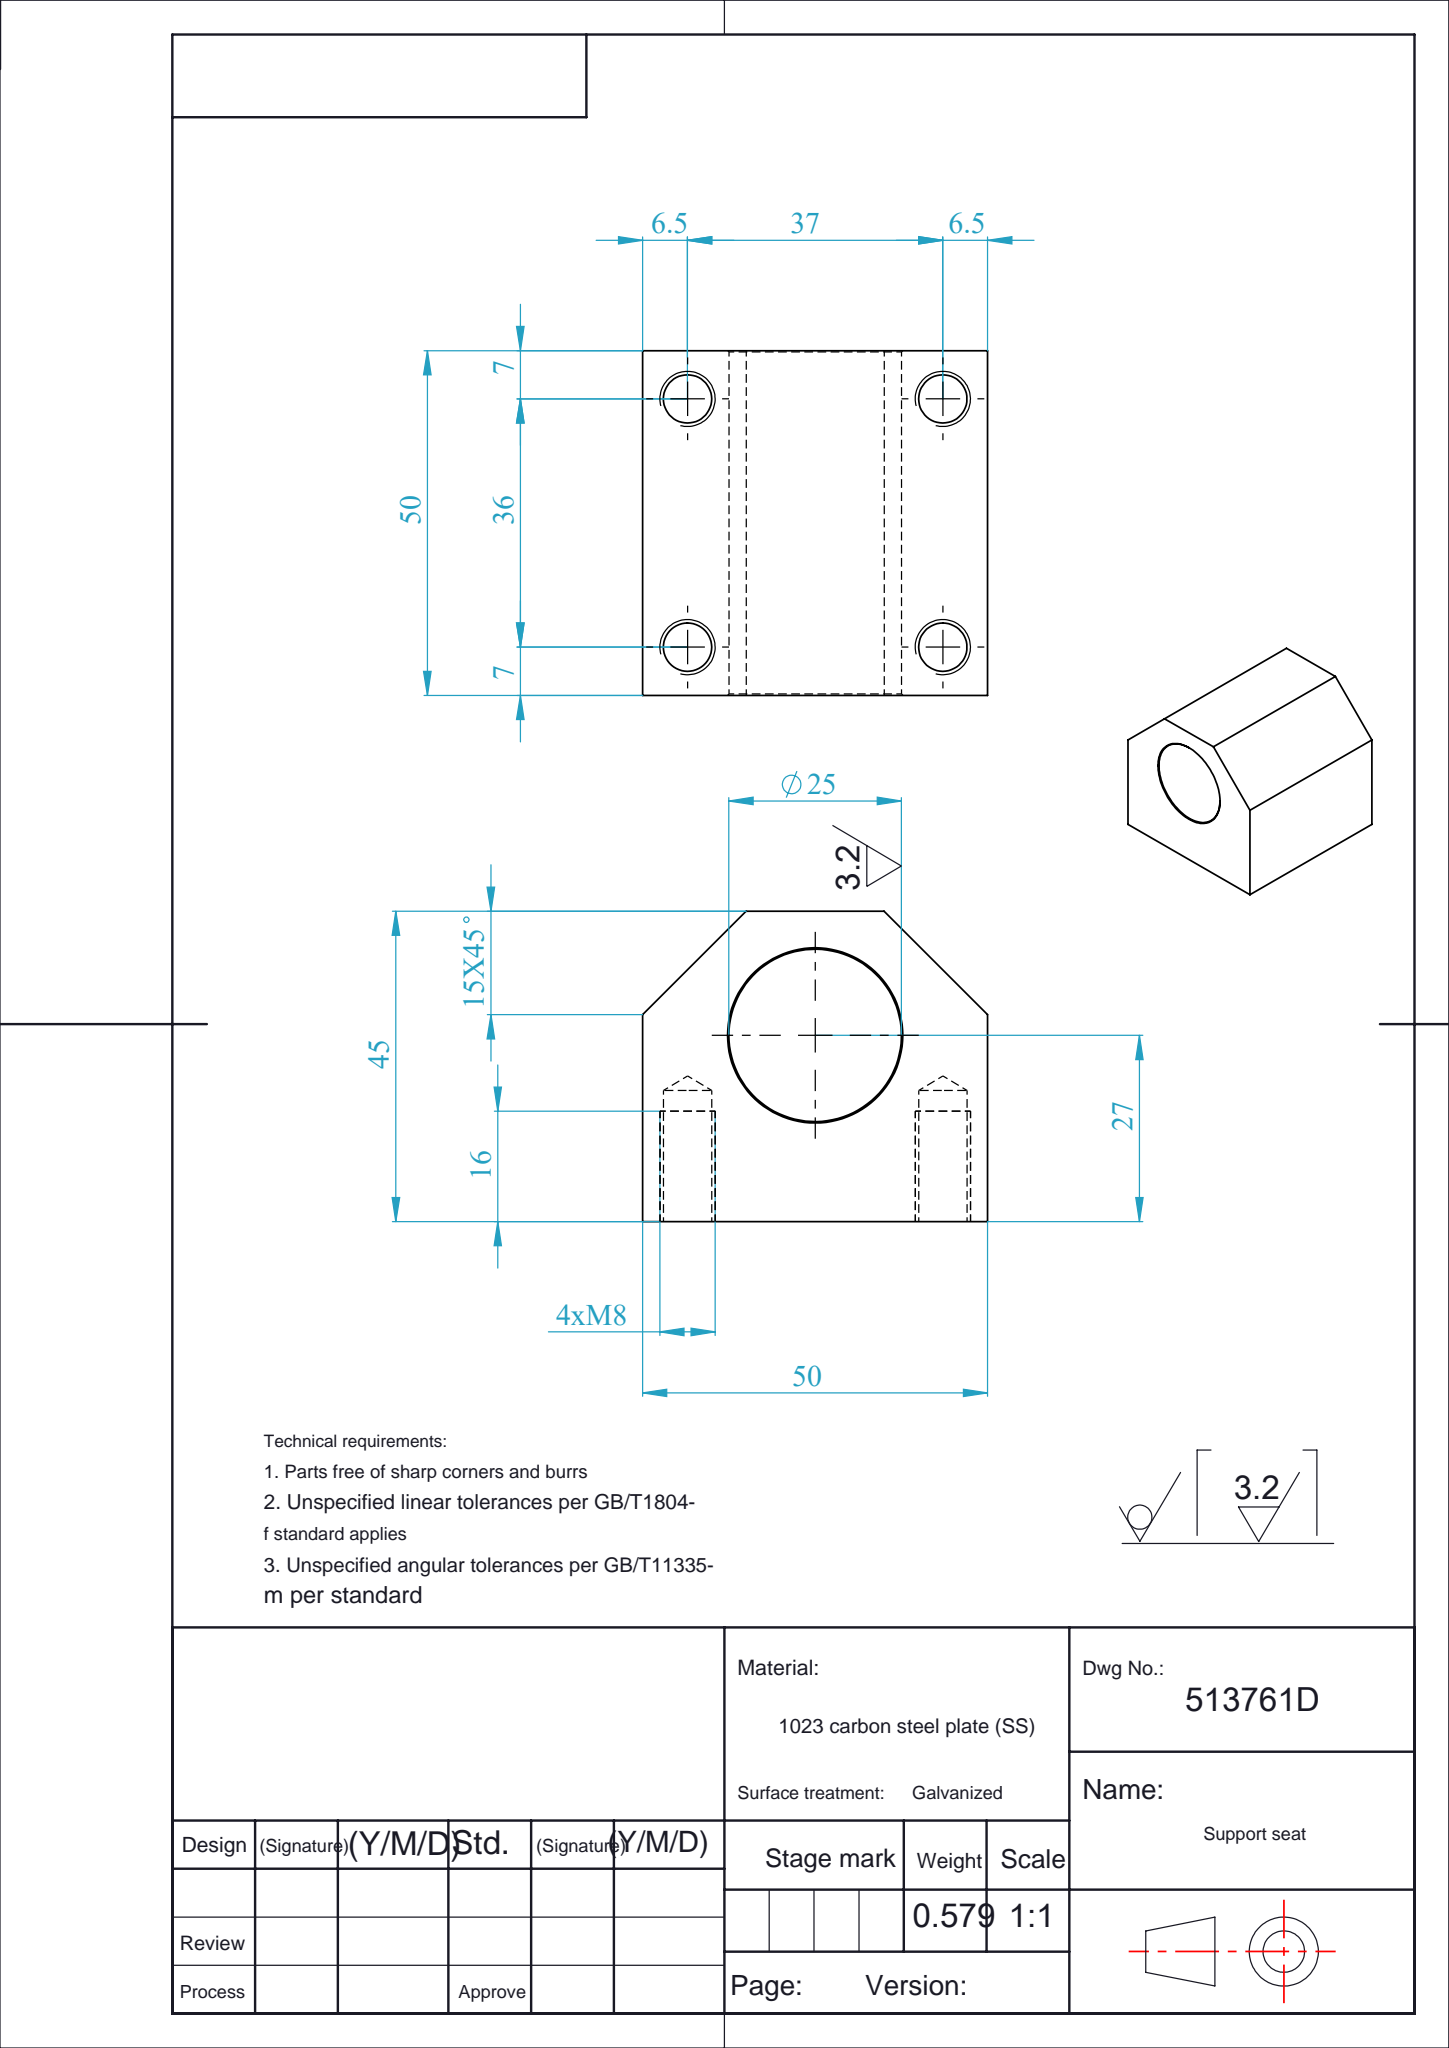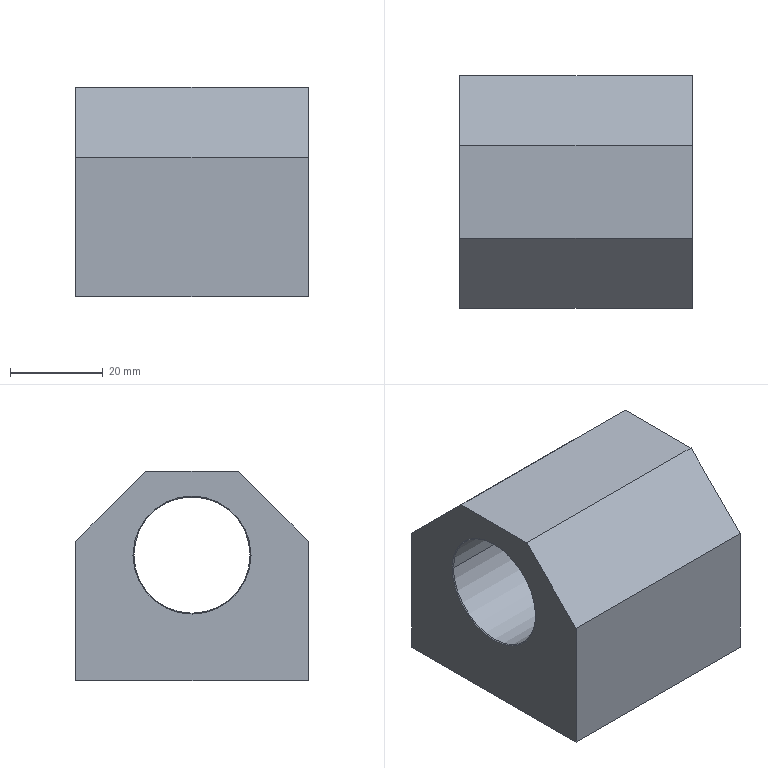Part | SolidWorks | features Chamfer 3, Extrusion 1, HoleWzd 1, ICE 1 | 1 solid | 30 faces | box 50 x 50 x 45 mm | volume 73670 mm3 | cone 12 | cylinder 10 | plane 8 | commonest cylinder face diameters 7 x8 25 x2
STEP:
#1=CARTESIAN_POINT('',(-24.8,12.5,27.));
#2=VERTEX_POINT('',#1);
#3=CARTESIAN_POINT('',(-24.8,-12.5,27.));
#4=VERTEX_POINT('',#3);
#5=CARTESIAN_POINT('',(-24.8,0.,27.));
#6=DIRECTION('',(-1.,0.,0.));
#7=DIRECTION('',(0.,1.,0.));
#8=AXIS2_PLACEMENT_3D('',#5,#6,#7);
#9=CIRCLE('',#8,12.5);
#10=EDGE_CURVE('',#2,#4,#9,.T.);
#11=ORIENTED_EDGE('',*,*,#10,.F.);
#12=CARTESIAN_POINT('',(-25.,12.7,27.));
#13=VERTEX_POINT('',#12);
#14=CARTESIAN_POINT('',(-25.,12.7,27.));
#15=DIRECTION('',(-0.7071,0.7071,0.));
#16=VECTOR('',#15,1000.);
#17=LINE('',#14,#16);
#18=EDGE_CURVE('',#2,#13,#17,.T.);
#19=ORIENTED_EDGE('',*,*,#18,.T.);
#20=CARTESIAN_POINT('',(-25.,-12.7,27.));
#21=VERTEX_POINT('',#20);
#22=CARTESIAN_POINT('',(-25.,0.,27.));
#23=DIRECTION('',(1.,0.,0.));
#24=DIRECTION('',(0.,1.,0.));
#25=AXIS2_PLACEMENT_3D('',#22,#23,#24);
#26=CIRCLE('',#25,12.7);
#27=EDGE_CURVE('',#21,#13,#26,.T.);
#28=ORIENTED_EDGE('',*,*,#27,.F.);
#29=CARTESIAN_POINT('',(-25.,-12.7,27.));
#30=DIRECTION('',(-0.7071,-0.7071,0.));
#31=VECTOR('',#30,1000.);
#32=LINE('',#29,#31);
#33=EDGE_CURVE('',#4,#21,#32,.T.);
#34=ORIENTED_EDGE('',*,*,#33,.F.);
#35=EDGE_LOOP('',(#11,#19,#28,#34));
#36=FACE_OUTER_BOUND('',#35,.T.);
#37=CARTESIAN_POINT('',(-25.,0.,27.));
#38=DIRECTION('',(-1.,0.,0.));
#39=DIRECTION('',(0.,-1.,0.));
#40=AXIS2_PLACEMENT_3D('',#37,#38,#39);
#41=CONICAL_SURFACE('',#40,12.7,0.7854);
#42=ADVANCED_FACE('',(#36),#41,.F.);
#43=CARTESIAN_POINT('',(24.8,-12.5,27.));
#44=VERTEX_POINT('',#43);
#45=CARTESIAN_POINT('',(24.8,12.5,27.));
#46=VERTEX_POINT('',#45);
#47=CARTESIAN_POINT('',(24.8,0.,27.));
#48=DIRECTION('',(1.,0.,0.));
#49=DIRECTION('',(0.,-1.,0.));
#50=AXIS2_PLACEMENT_3D('',#47,#48,#49);
#51=CIRCLE('',#50,12.5);
#52=EDGE_CURVE('',#44,#46,#51,.T.);
#53=ORIENTED_EDGE('',*,*,#52,.F.);
#54=CARTESIAN_POINT('',(25.,-12.7,27.));
#55=VERTEX_POINT('',#54);
#56=CARTESIAN_POINT('',(24.8,-12.5,27.));
#57=DIRECTION('',(0.7071,-0.7071,0.));
#58=VECTOR('',#57,1000.);
#59=LINE('',#56,#58);
#60=EDGE_CURVE('',#44,#55,#59,.T.);
#61=ORIENTED_EDGE('',*,*,#60,.T.);
#62=CARTESIAN_POINT('',(25.,12.7,27.));
#63=VERTEX_POINT('',#62);
#64=CARTESIAN_POINT('',(25.,0.,27.));
#65=DIRECTION('',(-1.,0.,0.));
#66=DIRECTION('',(0.,-1.,0.));
#67=AXIS2_PLACEMENT_3D('',#64,#65,#66);
#68=CIRCLE('',#67,12.7);
#69=EDGE_CURVE('',#63,#55,#68,.T.);
#70=ORIENTED_EDGE('',*,*,#69,.F.);
#71=CARTESIAN_POINT('',(24.8,12.5,27.));
#72=DIRECTION('',(0.7071,0.7071,0.));
#73=VECTOR('',#72,1000.);
#74=LINE('',#71,#73);
#75=EDGE_CURVE('',#46,#63,#74,.T.);
#76=ORIENTED_EDGE('',*,*,#75,.F.);
#77=EDGE_LOOP('',(#53,#61,#70,#76));
#78=FACE_OUTER_BOUND('',#77,.T.);
#79=CARTESIAN_POINT('',(24.8,0.,27.));
#80=DIRECTION('',(1.,0.,0.));
#81=DIRECTION('',(0.,1.,0.));
#82=AXIS2_PLACEMENT_3D('',#79,#80,#81);
#83=CONICAL_SURFACE('',#82,12.5,0.7854);
#84=ADVANCED_FACE('',(#78),#83,.F.);
#85=CARTESIAN_POINT('',(21.5,18.5,19.));
#86=VERTEX_POINT('',#85);
#87=CARTESIAN_POINT('',(14.5,18.5,19.));
#88=VERTEX_POINT('',#87);
#89=CARTESIAN_POINT('',(18.,18.5,19.));
#90=DIRECTION('',(0.,0.,-1.));
#91=DIRECTION('',(-1.,0.,0.));
#92=AXIS2_PLACEMENT_3D('',#89,#90,#91);
#93=CIRCLE('',#92,3.5);
#94=EDGE_CURVE('',#86,#88,#93,.T.);
#95=ORIENTED_EDGE('',*,*,#94,.F.);
#96=CARTESIAN_POINT('',(21.5,18.5,0.));
#97=VERTEX_POINT('',#96);
#98=CARTESIAN_POINT('',(21.5,18.5,0.));
#99=DIRECTION('',(0.,0.,-1.));
#100=VECTOR('',#99,1000.);
#101=LINE('',#98,#100);
#102=EDGE_CURVE('',#86,#97,#101,.T.);
#103=ORIENTED_EDGE('',*,*,#102,.T.);
#104=CARTESIAN_POINT('',(14.5,18.5,0.));
#105=VERTEX_POINT('',#104);
#106=CARTESIAN_POINT('',(18.,18.5,0.));
#107=DIRECTION('',(0.,0.,-1.));
#108=DIRECTION('',(-1.,0.,0.));
#109=AXIS2_PLACEMENT_3D('',#106,#107,#108);
#110=CIRCLE('',#109,3.5);
#111=EDGE_CURVE('',#97,#105,#110,.T.);
#112=ORIENTED_EDGE('',*,*,#111,.T.);
#113=CARTESIAN_POINT('',(14.5,18.5,0.));
#114=DIRECTION('',(0.,0.,-1.));
#115=VECTOR('',#114,1000.);
#116=LINE('',#113,#115);
#117=EDGE_CURVE('',#88,#105,#116,.T.);
#118=ORIENTED_EDGE('',*,*,#117,.F.);
#119=EDGE_LOOP('',(#95,#103,#112,#118));
#120=FACE_OUTER_BOUND('',#119,.T.);
#121=CARTESIAN_POINT('',(18.,18.5,0.));
#122=DIRECTION('',(0.,0.,-1.));
#123=DIRECTION('',(-1.,0.,0.));
#124=AXIS2_PLACEMENT_3D('',#121,#122,#123);
#125=CYLINDRICAL_SURFACE('',#124,3.5);
#126=ADVANCED_FACE('',(#120),#125,.F.);
#127=CARTESIAN_POINT('',(18.,18.5,21.103));
#128=VERTEX_POINT('',#127);
#129=CARTESIAN_POINT('',(14.5,18.5,19.));
#130=DIRECTION('',(-0.8572,0.,-0.515));
#131=VECTOR('',#130,1000.);
#132=LINE('',#129,#131);
#133=EDGE_CURVE('',#128,#88,#132,.T.);
#134=ORIENTED_EDGE('',*,*,#133,.F.);
#135=CARTESIAN_POINT('',(21.5,18.5,19.));
#136=DIRECTION('',(0.8572,0.,-0.515));
#137=VECTOR('',#136,1000.);
#138=LINE('',#135,#137);
#139=EDGE_CURVE('',#128,#86,#138,.T.);
#140=ORIENTED_EDGE('',*,*,#139,.T.);
#141=ORIENTED_EDGE('',*,*,#94,.T.);
#142=EDGE_LOOP('',(#134,#140,#141));
#143=FACE_OUTER_BOUND('',#142,.T.);
#144=CARTESIAN_POINT('',(18.,18.5,19.));
#145=DIRECTION('',(0.,0.,-1.));
#146=DIRECTION('',(-1.,0.,0.));
#147=AXIS2_PLACEMENT_3D('',#144,#145,#146);
#148=CONICAL_SURFACE('',#147,3.5,1.03);
#149=ADVANCED_FACE('',(#143),#148,.F.);
#150=CARTESIAN_POINT('',(-14.5,18.5,19.));
#151=VERTEX_POINT('',#150);
#152=CARTESIAN_POINT('',(-21.5,18.5,19.));
#153=VERTEX_POINT('',#152);
#154=CARTESIAN_POINT('',(-18.,18.5,19.));
#155=DIRECTION('',(0.,0.,-1.));
#156=DIRECTION('',(-1.,0.,0.));
#157=AXIS2_PLACEMENT_3D('',#154,#155,#156);
#158=CIRCLE('',#157,3.5);
#159=EDGE_CURVE('',#151,#153,#158,.T.);
#160=ORIENTED_EDGE('',*,*,#159,.F.);
#161=CARTESIAN_POINT('',(-14.5,18.5,0.));
#162=VERTEX_POINT('',#161);
#163=CARTESIAN_POINT('',(-14.5,18.5,0.));
#164=DIRECTION('',(0.,0.,-1.));
#165=VECTOR('',#164,1000.);
#166=LINE('',#163,#165);
#167=EDGE_CURVE('',#151,#162,#166,.T.);
#168=ORIENTED_EDGE('',*,*,#167,.T.);
#169=CARTESIAN_POINT('',(-21.5,18.5,0.));
#170=VERTEX_POINT('',#169);
#171=CARTESIAN_POINT('',(-18.,18.5,0.));
#172=DIRECTION('',(0.,0.,-1.));
#173=DIRECTION('',(-1.,0.,0.));
#174=AXIS2_PLACEMENT_3D('',#171,#172,#173);
#175=CIRCLE('',#174,3.5);
#176=EDGE_CURVE('',#162,#170,#175,.T.);
#177=ORIENTED_EDGE('',*,*,#176,.T.);
#178=CARTESIAN_POINT('',(-21.5,18.5,0.));
#179=DIRECTION('',(0.,0.,-1.));
#180=VECTOR('',#179,1000.);
#181=LINE('',#178,#180);
#182=EDGE_CURVE('',#153,#170,#181,.T.);
#183=ORIENTED_EDGE('',*,*,#182,.F.);
#184=EDGE_LOOP('',(#160,#168,#177,#183));
#185=FACE_OUTER_BOUND('',#184,.T.);
#186=CARTESIAN_POINT('',(-18.,18.5,0.));
#187=DIRECTION('',(0.,0.,-1.));
#188=DIRECTION('',(-1.,0.,0.));
#189=AXIS2_PLACEMENT_3D('',#186,#187,#188);
#190=CYLINDRICAL_SURFACE('',#189,3.5);
#191=ADVANCED_FACE('',(#185),#190,.F.);
#192=CARTESIAN_POINT('',(-18.,18.5,21.103));
#193=VERTEX_POINT('',#192);
#194=CARTESIAN_POINT('',(-21.5,18.5,19.));
#195=DIRECTION('',(-0.8572,0.,-0.515));
#196=VECTOR('',#195,1000.);
#197=LINE('',#194,#196);
#198=EDGE_CURVE('',#193,#153,#197,.T.);
#199=ORIENTED_EDGE('',*,*,#198,.F.);
#200=CARTESIAN_POINT('',(-14.5,18.5,19.));
#201=DIRECTION('',(0.8572,0.,-0.515));
#202=VECTOR('',#201,1000.);
#203=LINE('',#200,#202);
#204=EDGE_CURVE('',#193,#151,#203,.T.);
#205=ORIENTED_EDGE('',*,*,#204,.T.);
#206=ORIENTED_EDGE('',*,*,#159,.T.);
#207=EDGE_LOOP('',(#199,#205,#206));
#208=FACE_OUTER_BOUND('',#207,.T.);
#209=CARTESIAN_POINT('',(-18.,18.5,19.));
#210=DIRECTION('',(0.,0.,-1.));
#211=DIRECTION('',(-1.,0.,0.));
#212=AXIS2_PLACEMENT_3D('',#209,#210,#211);
#213=CONICAL_SURFACE('',#212,3.5,1.03);
#214=ADVANCED_FACE('',(#208),#213,.F.);
#215=CARTESIAN_POINT('',(-14.5,-18.5,19.));
#216=VERTEX_POINT('',#215);
#217=CARTESIAN_POINT('',(-21.5,-18.5,19.));
#218=VERTEX_POINT('',#217);
#219=CARTESIAN_POINT('',(-18.,-18.5,19.));
#220=DIRECTION('',(0.,0.,-1.));
#221=DIRECTION('',(-1.,0.,0.));
#222=AXIS2_PLACEMENT_3D('',#219,#220,#221);
#223=CIRCLE('',#222,3.5);
#224=EDGE_CURVE('',#216,#218,#223,.T.);
#225=ORIENTED_EDGE('',*,*,#224,.F.);
#226=CARTESIAN_POINT('',(-14.5,-18.5,0.));
#227=VERTEX_POINT('',#226);
#228=CARTESIAN_POINT('',(-14.5,-18.5,0.));
#229=DIRECTION('',(0.,0.,-1.));
#230=VECTOR('',#229,1000.);
#231=LINE('',#228,#230);
#232=EDGE_CURVE('',#216,#227,#231,.T.);
#233=ORIENTED_EDGE('',*,*,#232,.T.);
#234=CARTESIAN_POINT('',(-21.5,-18.5,0.));
#235=VERTEX_POINT('',#234);
#236=CARTESIAN_POINT('',(-18.,-18.5,0.));
#237=DIRECTION('',(0.,0.,-1.));
#238=DIRECTION('',(-1.,0.,0.));
#239=AXIS2_PLACEMENT_3D('',#236,#237,#238);
#240=CIRCLE('',#239,3.5);
#241=EDGE_CURVE('',#227,#235,#240,.T.);
#242=ORIENTED_EDGE('',*,*,#241,.T.);
#243=CARTESIAN_POINT('',(-21.5,-18.5,0.));
#244=DIRECTION('',(0.,0.,-1.));
#245=VECTOR('',#244,1000.);
#246=LINE('',#243,#245);
#247=EDGE_CURVE('',#218,#235,#246,.T.);
#248=ORIENTED_EDGE('',*,*,#247,.F.);
#249=EDGE_LOOP('',(#225,#233,#242,#248));
#250=FACE_OUTER_BOUND('',#249,.T.);
#251=CARTESIAN_POINT('',(-18.,-18.5,0.));
#252=DIRECTION('',(0.,0.,-1.));
#253=DIRECTION('',(-1.,0.,0.));
#254=AXIS2_PLACEMENT_3D('',#251,#252,#253);
#255=CYLINDRICAL_SURFACE('',#254,3.5);
#256=ADVANCED_FACE('',(#250),#255,.F.);
#257=CARTESIAN_POINT('',(-18.,-18.5,21.103));
#258=VERTEX_POINT('',#257);
#259=CARTESIAN_POINT('',(-21.5,-18.5,19.));
#260=DIRECTION('',(-0.8572,0.,-0.515));
#261=VECTOR('',#260,1000.);
#262=LINE('',#259,#261);
#263=EDGE_CURVE('',#258,#218,#262,.T.);
#264=ORIENTED_EDGE('',*,*,#263,.F.);
#265=CARTESIAN_POINT('',(-14.5,-18.5,19.));
#266=DIRECTION('',(0.8572,0.,-0.515));
#267=VECTOR('',#266,1000.);
#268=LINE('',#265,#267);
#269=EDGE_CURVE('',#258,#216,#268,.T.);
#270=ORIENTED_EDGE('',*,*,#269,.T.);
#271=ORIENTED_EDGE('',*,*,#224,.T.);
#272=EDGE_LOOP('',(#264,#270,#271));
#273=FACE_OUTER_BOUND('',#272,.T.);
#274=CARTESIAN_POINT('',(-18.,-18.5,19.));
#275=DIRECTION('',(0.,0.,-1.));
#276=DIRECTION('',(-1.,0.,0.));
#277=AXIS2_PLACEMENT_3D('',#274,#275,#276);
#278=CONICAL_SURFACE('',#277,3.5,1.03);
#279=ADVANCED_FACE('',(#273),#278,.F.);
#280=CARTESIAN_POINT('',(21.5,-18.5,19.));
#281=VERTEX_POINT('',#280);
#282=CARTESIAN_POINT('',(14.5,-18.5,19.));
#283=VERTEX_POINT('',#282);
#284=CARTESIAN_POINT('',(18.,-18.5,19.));
#285=DIRECTION('',(0.,0.,-1.));
#286=DIRECTION('',(-1.,0.,0.));
#287=AXIS2_PLACEMENT_3D('',#284,#285,#286);
#288=CIRCLE('',#287,3.5);
#289=EDGE_CURVE('',#281,#283,#288,.T.);
#290=ORIENTED_EDGE('',*,*,#289,.F.);
#291=CARTESIAN_POINT('',(21.5,-18.5,0.));
#292=VERTEX_POINT('',#291);
#293=CARTESIAN_POINT('',(21.5,-18.5,0.));
#294=DIRECTION('',(0.,0.,-1.));
#295=VECTOR('',#294,1000.);
#296=LINE('',#293,#295);
#297=EDGE_CURVE('',#281,#292,#296,.T.);
#298=ORIENTED_EDGE('',*,*,#297,.T.);
#299=CARTESIAN_POINT('',(14.5,-18.5,0.));
#300=VERTEX_POINT('',#299);
#301=CARTESIAN_POINT('',(18.,-18.5,0.));
#302=DIRECTION('',(0.,0.,-1.));
#303=DIRECTION('',(-1.,0.,0.));
#304=AXIS2_PLACEMENT_3D('',#301,#302,#303);
#305=CIRCLE('',#304,3.5);
#306=EDGE_CURVE('',#292,#300,#305,.T.);
#307=ORIENTED_EDGE('',*,*,#306,.T.);
#308=CARTESIAN_POINT('',(14.5,-18.5,0.));
#309=DIRECTION('',(0.,0.,-1.));
#310=VECTOR('',#309,1000.);
#311=LINE('',#308,#310);
#312=EDGE_CURVE('',#283,#300,#311,.T.);
#313=ORIENTED_EDGE('',*,*,#312,.F.);
#314=EDGE_LOOP('',(#290,#298,#307,#313));
#315=FACE_OUTER_BOUND('',#314,.T.);
#316=CARTESIAN_POINT('',(18.,-18.5,0.));
#317=DIRECTION('',(0.,0.,-1.));
#318=DIRECTION('',(-1.,0.,0.));
#319=AXIS2_PLACEMENT_3D('',#316,#317,#318);
#320=CYLINDRICAL_SURFACE('',#319,3.5);
#321=ADVANCED_FACE('',(#315),#320,.F.);
#322=CARTESIAN_POINT('',(18.,-18.5,21.103));
#323=VERTEX_POINT('',#322);
#324=CARTESIAN_POINT('',(14.5,-18.5,19.));
#325=DIRECTION('',(-0.8572,0.,-0.515));
#326=VECTOR('',#325,1000.);
#327=LINE('',#324,#326);
#328=EDGE_CURVE('',#323,#283,#327,.T.);
#329=ORIENTED_EDGE('',*,*,#328,.F.);
#330=CARTESIAN_POINT('',(21.5,-18.5,19.));
#331=DIRECTION('',(0.8572,0.,-0.515));
#332=VECTOR('',#331,1000.);
#333=LINE('',#330,#332);
#334=EDGE_CURVE('',#323,#281,#333,.T.);
#335=ORIENTED_EDGE('',*,*,#334,.T.);
#336=ORIENTED_EDGE('',*,*,#289,.T.);
#337=EDGE_LOOP('',(#329,#335,#336));
#338=FACE_OUTER_BOUND('',#337,.T.);
#339=CARTESIAN_POINT('',(18.,-18.5,19.));
#340=DIRECTION('',(0.,0.,-1.));
#341=DIRECTION('',(-1.,0.,0.));
#342=AXIS2_PLACEMENT_3D('',#339,#340,#341);
#343=CONICAL_SURFACE('',#342,3.5,1.03);
#344=ADVANCED_FACE('',(#338),#343,.F.);
#345=ORIENTED_EDGE('',*,*,#10,.T.);
#346=CARTESIAN_POINT('',(-31.,-12.5,27.));
#347=DIRECTION('',(1.,0.,0.));
#348=VECTOR('',#347,1000.);
#349=LINE('',#346,#348);
#350=EDGE_CURVE('',#4,#44,#349,.T.);
#351=ORIENTED_EDGE('',*,*,#350,.T.);
#352=ORIENTED_EDGE('',*,*,#52,.T.);
#353=CARTESIAN_POINT('',(-31.,12.5,27.));
#354=DIRECTION('',(1.,0.,0.));
#355=VECTOR('',#354,1000.);
#356=LINE('',#353,#355);
#357=EDGE_CURVE('',#2,#46,#356,.T.);
#358=ORIENTED_EDGE('',*,*,#357,.F.);
#359=EDGE_LOOP('',(#345,#351,#352,#358));
#360=FACE_OUTER_BOUND('',#359,.T.);
#361=CARTESIAN_POINT('',(-31.,0.,27.));
#362=DIRECTION('',(1.,0.,0.));
#363=DIRECTION('',(0.,1.,0.));
#364=AXIS2_PLACEMENT_3D('',#361,#362,#363);
#365=CYLINDRICAL_SURFACE('',#364,12.5);
#366=ADVANCED_FACE('',(#360),#365,.F.);
#367=ORIENTED_EDGE('',*,*,#69,.T.);
#368=CARTESIAN_POINT('',(25.,0.,27.));
#369=DIRECTION('',(-1.,0.,0.));
#370=DIRECTION('',(0.,-1.,0.));
#371=AXIS2_PLACEMENT_3D('',#368,#369,#370);
#372=CIRCLE('',#371,12.7);
#373=EDGE_CURVE('',#55,#63,#372,.T.);
#374=ORIENTED_EDGE('',*,*,#373,.T.);
#375=EDGE_LOOP('',(#367,#374));
#376=FACE_BOUND('',#375,.T.);
#377=CARTESIAN_POINT('',(25.,25.,30.));
#378=VERTEX_POINT('',#377);
#379=CARTESIAN_POINT('',(25.,25.,0.));
#380=VERTEX_POINT('',#379);
#381=CARTESIAN_POINT('',(25.,25.,45.));
#382=DIRECTION('',(0.,0.,-1.));
#383=VECTOR('',#382,1000.);
#384=LINE('',#381,#383);
#385=EDGE_CURVE('',#378,#380,#384,.T.);
#386=ORIENTED_EDGE('',*,*,#385,.F.);
#387=CARTESIAN_POINT('',(25.,10.,45.));
#388=VERTEX_POINT('',#387);
#389=CARTESIAN_POINT('',(25.,10.,45.));
#390=DIRECTION('',(0.,-0.7071,0.7071));
#391=VECTOR('',#390,1000.);
#392=LINE('',#389,#391);
#393=EDGE_CURVE('',#378,#388,#392,.T.);
#394=ORIENTED_EDGE('',*,*,#393,.T.);
#395=CARTESIAN_POINT('',(25.,-10.,45.));
#396=VERTEX_POINT('',#395);
#397=CARTESIAN_POINT('',(25.,25.,45.));
#398=DIRECTION('',(0.,1.,0.));
#399=VECTOR('',#398,1000.);
#400=LINE('',#397,#399);
#401=EDGE_CURVE('',#396,#388,#400,.T.);
#402=ORIENTED_EDGE('',*,*,#401,.F.);
#403=CARTESIAN_POINT('',(25.,-25.,30.));
#404=VERTEX_POINT('',#403);
#405=CARTESIAN_POINT('',(25.,-10.,45.));
#406=DIRECTION('',(0.,-0.7071,-0.7071));
#407=VECTOR('',#406,1000.);
#408=LINE('',#405,#407);
#409=EDGE_CURVE('',#396,#404,#408,.T.);
#410=ORIENTED_EDGE('',*,*,#409,.T.);
#411=CARTESIAN_POINT('',(25.,-25.,0.));
#412=VERTEX_POINT('',#411);
#413=CARTESIAN_POINT('',(25.,-25.,45.));
#414=DIRECTION('',(0.,0.,-1.));
#415=VECTOR('',#414,1000.);
#416=LINE('',#413,#415);
#417=EDGE_CURVE('',#404,#412,#416,.T.);
#418=ORIENTED_EDGE('',*,*,#417,.T.);
#419=CARTESIAN_POINT('',(25.,25.,0.));
#420=DIRECTION('',(0.,1.,0.));
#421=VECTOR('',#420,1000.);
#422=LINE('',#419,#421);
#423=EDGE_CURVE('',#412,#380,#422,.T.);
#424=ORIENTED_EDGE('',*,*,#423,.T.);
#425=EDGE_LOOP('',(#386,#394,#402,#410,#418,#424));
#426=FACE_OUTER_BOUND('',#425,.T.);
#427=CARTESIAN_POINT('',(25.,25.,45.));
#428=DIRECTION('',(-1.,0.,0.));
#429=DIRECTION('',(0.,-1.,0.));
#430=AXIS2_PLACEMENT_3D('',#427,#428,#429);
#431=PLANE('',#430);
#432=ADVANCED_FACE('',(#376,#426),#431,.F.);
#433=CARTESIAN_POINT('',(-25.,25.,30.));
#434=VERTEX_POINT('',#433);
#435=CARTESIAN_POINT('',(-25.,25.,0.));
#436=VERTEX_POINT('',#435);
#437=CARTESIAN_POINT('',(-25.,25.,45.));
#438=DIRECTION('',(0.,0.,-1.));
#439=VECTOR('',#438,1000.);
#440=LINE('',#437,#439);
#441=EDGE_CURVE('',#434,#436,#440,.T.);
#442=ORIENTED_EDGE('',*,*,#441,.F.);
#443=CARTESIAN_POINT('',(25.,25.,30.));
#444=DIRECTION('',(1.,0.,0.));
#445=VECTOR('',#444,1000.);
#446=LINE('',#443,#445);
#447=EDGE_CURVE('',#434,#378,#446,.T.);
#448=ORIENTED_EDGE('',*,*,#447,.T.);
#449=ORIENTED_EDGE('',*,*,#385,.T.);
#450=CARTESIAN_POINT('',(-25.,25.,0.));
#451=DIRECTION('',(-1.,0.,0.));
#452=VECTOR('',#451,1000.);
#453=LINE('',#450,#452);
#454=EDGE_CURVE('',#380,#436,#453,.T.);
#455=ORIENTED_EDGE('',*,*,#454,.T.);
#456=EDGE_LOOP('',(#442,#448,#449,#455));
#457=FACE_OUTER_BOUND('',#456,.T.);
#458=CARTESIAN_POINT('',(-25.,25.,45.));
#459=DIRECTION('',(0.,-1.,0.));
#460=DIRECTION('',(0.,0.,-1.));
#461=AXIS2_PLACEMENT_3D('',#458,#459,#460);
#462=PLANE('',#461);
#463=ADVANCED_FACE('',(#457),#462,.F.);
#464=ORIENTED_EDGE('',*,*,#27,.T.);
#465=CARTESIAN_POINT('',(-25.,0.,27.));
#466=DIRECTION('',(1.,0.,0.));
#467=DIRECTION('',(0.,1.,0.));
#468=AXIS2_PLACEMENT_3D('',#465,#466,#467);
#469=CIRCLE('',#468,12.7);
#470=EDGE_CURVE('',#13,#21,#469,.T.);
#471=ORIENTED_EDGE('',*,*,#470,.T.);
#472=EDGE_LOOP('',(#464,#471));
#473=FACE_BOUND('',#472,.T.);
#474=CARTESIAN_POINT('',(-25.,10.,45.));
#475=VERTEX_POINT('',#474);
#476=CARTESIAN_POINT('',(-25.,-10.,45.));
#477=VERTEX_POINT('',#476);
#478=CARTESIAN_POINT('',(-25.,25.,45.));
#479=DIRECTION('',(0.,-1.,0.));
#480=VECTOR('',#479,1000.);
#481=LINE('',#478,#480);
#482=EDGE_CURVE('',#475,#477,#481,.T.);
#483=ORIENTED_EDGE('',*,*,#482,.F.);
#484=CARTESIAN_POINT('',(-25.,10.,45.));
#485=DIRECTION('',(0.,0.7071,-0.7071));
#486=VECTOR('',#485,1000.);
#487=LINE('',#484,#486);
#488=EDGE_CURVE('',#475,#434,#487,.T.);
#489=ORIENTED_EDGE('',*,*,#488,.T.);
#490=ORIENTED_EDGE('',*,*,#441,.T.);
#491=CARTESIAN_POINT('',(-25.,-25.,0.));
#492=VERTEX_POINT('',#491);
#493=CARTESIAN_POINT('',(-25.,25.,0.));
#494=DIRECTION('',(0.,-1.,0.));
#495=VECTOR('',#494,1000.);
#496=LINE('',#493,#495);
#497=EDGE_CURVE('',#436,#492,#496,.T.);
#498=ORIENTED_EDGE('',*,*,#497,.T.);
#499=CARTESIAN_POINT('',(-25.,-25.,30.));
#500=VERTEX_POINT('',#499);
#501=CARTESIAN_POINT('',(-25.,-25.,45.));
#502=DIRECTION('',(0.,0.,-1.));
#503=VECTOR('',#502,1000.);
#504=LINE('',#501,#503);
#505=EDGE_CURVE('',#500,#492,#504,.T.);
#506=ORIENTED_EDGE('',*,*,#505,.F.);
#507=CARTESIAN_POINT('',(-25.,-10.,45.));
#508=DIRECTION('',(0.,0.7071,0.7071));
#509=VECTOR('',#508,1000.);
#510=LINE('',#507,#509);
#511=EDGE_CURVE('',#500,#477,#510,.T.);
#512=ORIENTED_EDGE('',*,*,#511,.T.);
#513=EDGE_LOOP('',(#483,#489,#490,#498,#506,#512));
#514=FACE_OUTER_BOUND('',#513,.T.);
#515=CARTESIAN_POINT('',(-25.,25.,45.));
#516=DIRECTION('',(1.,0.,0.));
#517=DIRECTION('',(0.,1.,0.));
#518=AXIS2_PLACEMENT_3D('',#515,#516,#517);
#519=PLANE('',#518);
#520=ADVANCED_FACE('',(#473,#514),#519,.F.);
#521=ORIENTED_EDGE('',*,*,#417,.F.);
#522=CARTESIAN_POINT('',(-25.,-25.,30.));
#523=DIRECTION('',(-1.,0.,0.));
#524=VECTOR('',#523,1000.);
#525=LINE('',#522,#524);
#526=EDGE_CURVE('',#404,#500,#525,.T.);
#527=ORIENTED_EDGE('',*,*,#526,.T.);
#528=ORIENTED_EDGE('',*,*,#505,.T.);
#529=CARTESIAN_POINT('',(-25.,-25.,0.));
#530=DIRECTION('',(1.,0.,0.));
#531=VECTOR('',#530,1000.);
#532=LINE('',#529,#531);
#533=EDGE_CURVE('',#492,#412,#532,.T.);
#534=ORIENTED_EDGE('',*,*,#533,.T.);
#535=EDGE_LOOP('',(#521,#527,#528,#534));
#536=FACE_OUTER_BOUND('',#535,.T.);
#537=CARTESIAN_POINT('',(-25.,-25.,45.));
#538=DIRECTION('',(0.,1.,0.));
#539=DIRECTION('',(0.,0.,1.));
#540=AXIS2_PLACEMENT_3D('',#537,#538,#539);
#541=PLANE('',#540);
#542=ADVANCED_FACE('',(#536),#541,.F.);
#543=ORIENTED_EDGE('',*,*,#401,.T.);
#544=CARTESIAN_POINT('',(-25.,10.,45.));
#545=DIRECTION('',(-1.,0.,0.));
#546=VECTOR('',#545,1000.);
#547=LINE('',#544,#546);
#548=EDGE_CURVE('',#388,#475,#547,.T.);
#549=ORIENTED_EDGE('',*,*,#548,.T.);
#550=ORIENTED_EDGE('',*,*,#482,.T.);
#551=CARTESIAN_POINT('',(25.,-10.,45.));
#552=DIRECTION('',(1.,0.,0.));
#553=VECTOR('',#552,1000.);
#554=LINE('',#551,#553);
#555=EDGE_CURVE('',#477,#396,#554,.T.);
#556=ORIENTED_EDGE('',*,*,#555,.T.);
#557=EDGE_LOOP('',(#543,#549,#550,#556));
#558=FACE_OUTER_BOUND('',#557,.T.);
#559=CARTESIAN_POINT('',(0.,0.,45.));
#560=DIRECTION('',(0.,0.,1.));
#561=DIRECTION('',(1.,0.,0.));
#562=AXIS2_PLACEMENT_3D('',#559,#560,#561);
#563=PLANE('',#562);
#564=ADVANCED_FACE('',(#558),#563,.T.);
#565=CARTESIAN_POINT('',(18.,18.5,0.));
#566=DIRECTION('',(0.,0.,-1.));
#567=DIRECTION('',(-1.,0.,0.));
#568=AXIS2_PLACEMENT_3D('',#565,#566,#567);
#569=CIRCLE('',#568,3.5);
#570=EDGE_CURVE('',#105,#97,#569,.T.);
#571=ORIENTED_EDGE('',*,*,#570,.F.);
#572=ORIENTED_EDGE('',*,*,#111,.F.);
#573=EDGE_LOOP('',(#571,#572));
#574=FACE_BOUND('',#573,.T.);
#575=CARTESIAN_POINT('',(-18.,18.5,0.));
#576=DIRECTION('',(0.,0.,-1.));
#577=DIRECTION('',(-1.,0.,0.));
#578=AXIS2_PLACEMENT_3D('',#575,#576,#577);
#579=CIRCLE('',#578,3.5);
#580=EDGE_CURVE('',#170,#162,#579,.T.);
#581=ORIENTED_EDGE('',*,*,#580,.F.);
#582=ORIENTED_EDGE('',*,*,#176,.F.);
#583=EDGE_LOOP('',(#581,#582));
#584=FACE_BOUND('',#583,.T.);
#585=CARTESIAN_POINT('',(-18.,-18.5,0.));
#586=DIRECTION('',(0.,0.,-1.));
#587=DIRECTION('',(-1.,0.,0.));
#588=AXIS2_PLACEMENT_3D('',#585,#586,#587);
#589=CIRCLE('',#588,3.5);
#590=EDGE_CURVE('',#235,#227,#589,.T.);
#591=ORIENTED_EDGE('',*,*,#590,.F.);
#592=ORIENTED_EDGE('',*,*,#241,.F.);
#593=EDGE_LOOP('',(#591,#592));
#594=FACE_BOUND('',#593,.T.);
#595=CARTESIAN_POINT('',(18.,-18.5,0.));
#596=DIRECTION('',(0.,0.,-1.));
#597=DIRECTION('',(-1.,0.,0.));
#598=AXIS2_PLACEMENT_3D('',#595,#596,#597);
#599=CIRCLE('',#598,3.5);
#600=EDGE_CURVE('',#300,#292,#599,.T.);
#601=ORIENTED_EDGE('',*,*,#600,.F.);
#602=ORIENTED_EDGE('',*,*,#306,.F.);
#603=EDGE_LOOP('',(#601,#602));
#604=FACE_BOUND('',#603,.T.);
#605=ORIENTED_EDGE('',*,*,#423,.F.);
#606=ORIENTED_EDGE('',*,*,#533,.F.);
#607=ORIENTED_EDGE('',*,*,#497,.F.);
#608=ORIENTED_EDGE('',*,*,#454,.F.);
#609=EDGE_LOOP('',(#605,#606,#607,#608));
#610=FACE_OUTER_BOUND('',#609,.T.);
#611=CARTESIAN_POINT('',(0.,0.,0.));
#612=DIRECTION('',(0.,0.,1.));
#613=DIRECTION('',(1.,0.,0.));
#614=AXIS2_PLACEMENT_3D('',#611,#612,#613);
#615=PLANE('',#614);
#616=ADVANCED_FACE('',(#574,#584,#594,#604,#610),#615,.F.);
#617=ORIENTED_EDGE('',*,*,#350,.F.);
#618=CARTESIAN_POINT('',(-24.8,0.,27.));
#619=DIRECTION('',(-1.,0.,0.));
#620=DIRECTION('',(0.,1.,0.));
#621=AXIS2_PLACEMENT_3D('',#618,#619,#620);
#622=CIRCLE('',#621,12.5);
#623=EDGE_CURVE('',#4,#2,#622,.T.);
#624=ORIENTED_EDGE('',*,*,#623,.T.);
#625=ORIENTED_EDGE('',*,*,#357,.T.);
#626=CARTESIAN_POINT('',(24.8,0.,27.));
#627=DIRECTION('',(1.,0.,0.));
#628=DIRECTION('',(0.,-1.,0.));
#629=AXIS2_PLACEMENT_3D('',#626,#627,#628);
#630=CIRCLE('',#629,12.5);
#631=EDGE_CURVE('',#46,#44,#630,.T.);
#632=ORIENTED_EDGE('',*,*,#631,.T.);
#633=EDGE_LOOP('',(#617,#624,#625,#632));
#634=FACE_OUTER_BOUND('',#633,.T.);
#635=CARTESIAN_POINT('',(-31.,0.,27.));
#636=DIRECTION('',(1.,0.,0.));
#637=DIRECTION('',(0.,1.,0.));
#638=AXIS2_PLACEMENT_3D('',#635,#636,#637);
#639=CYLINDRICAL_SURFACE('',#638,12.5);
#640=ADVANCED_FACE('',(#634),#639,.F.);
#641=ORIENTED_EDGE('',*,*,#393,.F.);
#642=ORIENTED_EDGE('',*,*,#447,.F.);
#643=ORIENTED_EDGE('',*,*,#488,.F.);
#644=ORIENTED_EDGE('',*,*,#548,.F.);
#645=EDGE_LOOP('',(#641,#642,#643,#644));
#646=FACE_OUTER_BOUND('',#645,.T.);
#647=CARTESIAN_POINT('',(0.,10.,45.));
#648=DIRECTION('',(0.,0.7071,0.7071));
#649=DIRECTION('',(1.,0.,0.));
#650=AXIS2_PLACEMENT_3D('',#647,#648,#649);
#651=PLANE('',#650);
#652=ADVANCED_FACE('',(#646),#651,.T.);
#653=ORIENTED_EDGE('',*,*,#511,.F.);
#654=ORIENTED_EDGE('',*,*,#526,.F.);
#655=ORIENTED_EDGE('',*,*,#409,.F.);
#656=ORIENTED_EDGE('',*,*,#555,.F.);
#657=EDGE_LOOP('',(#653,#654,#655,#656));
#658=FACE_OUTER_BOUND('',#657,.T.);
#659=CARTESIAN_POINT('',(0.,-10.,45.));
#660=DIRECTION('',(0.,-0.7071,0.7071));
#661=DIRECTION('',(-1.,0.,0.));
#662=AXIS2_PLACEMENT_3D('',#659,#660,#661);
#663=PLANE('',#662);
#664=ADVANCED_FACE('',(#658),#663,.T.);
#665=ORIENTED_EDGE('',*,*,#334,.F.);
#666=ORIENTED_EDGE('',*,*,#328,.T.);
#667=CARTESIAN_POINT('',(18.,-18.5,19.));
#668=DIRECTION('',(0.,0.,-1.));
#669=DIRECTION('',(-1.,0.,0.));
#670=AXIS2_PLACEMENT_3D('',#667,#668,#669);
#671=CIRCLE('',#670,3.5);
#672=EDGE_CURVE('',#283,#281,#671,.T.);
#673=ORIENTED_EDGE('',*,*,#672,.T.);
#674=EDGE_LOOP('',(#665,#666,#673));
#675=FACE_OUTER_BOUND('',#674,.T.);
#676=CARTESIAN_POINT('',(18.,-18.5,19.));
#677=DIRECTION('',(0.,0.,-1.));
#678=DIRECTION('',(-1.,0.,0.));
#679=AXIS2_PLACEMENT_3D('',#676,#677,#678);
#680=CONICAL_SURFACE('',#679,3.5,1.03);
#681=ADVANCED_FACE('',(#675),#680,.F.);
#682=ORIENTED_EDGE('',*,*,#297,.F.);
#683=ORIENTED_EDGE('',*,*,#672,.F.);
#684=ORIENTED_EDGE('',*,*,#312,.T.);
#685=ORIENTED_EDGE('',*,*,#600,.T.);
#686=EDGE_LOOP('',(#682,#683,#684,#685));
#687=FACE_OUTER_BOUND('',#686,.T.);
#688=CARTESIAN_POINT('',(18.,-18.5,0.));
#689=DIRECTION('',(0.,0.,-1.));
#690=DIRECTION('',(-1.,0.,0.));
#691=AXIS2_PLACEMENT_3D('',#688,#689,#690);
#692=CYLINDRICAL_SURFACE('',#691,3.5);
#693=ADVANCED_FACE('',(#687),#692,.F.);
#694=ORIENTED_EDGE('',*,*,#269,.F.);
#695=ORIENTED_EDGE('',*,*,#263,.T.);
#696=CARTESIAN_POINT('',(-18.,-18.5,19.));
#697=DIRECTION('',(0.,0.,-1.));
#698=DIRECTION('',(-1.,0.,0.));
#699=AXIS2_PLACEMENT_3D('',#696,#697,#698);
#700=CIRCLE('',#699,3.5);
#701=EDGE_CURVE('',#218,#216,#700,.T.);
#702=ORIENTED_EDGE('',*,*,#701,.T.);
#703=EDGE_LOOP('',(#694,#695,#702));
#704=FACE_OUTER_BOUND('',#703,.T.);
#705=CARTESIAN_POINT('',(-18.,-18.5,19.));
#706=DIRECTION('',(0.,0.,-1.));
#707=DIRECTION('',(-1.,0.,0.));
#708=AXIS2_PLACEMENT_3D('',#705,#706,#707);
#709=CONICAL_SURFACE('',#708,3.5,1.03);
#710=ADVANCED_FACE('',(#704),#709,.F.);
#711=ORIENTED_EDGE('',*,*,#232,.F.);
#712=ORIENTED_EDGE('',*,*,#701,.F.);
#713=ORIENTED_EDGE('',*,*,#247,.T.);
#714=ORIENTED_EDGE('',*,*,#590,.T.);
#715=EDGE_LOOP('',(#711,#712,#713,#714));
#716=FACE_OUTER_BOUND('',#715,.T.);
#717=CARTESIAN_POINT('',(-18.,-18.5,0.));
#718=DIRECTION('',(0.,0.,-1.));
#719=DIRECTION('',(-1.,0.,0.));
#720=AXIS2_PLACEMENT_3D('',#717,#718,#719);
#721=CYLINDRICAL_SURFACE('',#720,3.5);
#722=ADVANCED_FACE('',(#716),#721,.F.);
#723=ORIENTED_EDGE('',*,*,#204,.F.);
#724=ORIENTED_EDGE('',*,*,#198,.T.);
#725=CARTESIAN_POINT('',(-18.,18.5,19.));
#726=DIRECTION('',(0.,0.,-1.));
#727=DIRECTION('',(-1.,0.,0.));
#728=AXIS2_PLACEMENT_3D('',#725,#726,#727);
#729=CIRCLE('',#728,3.5);
#730=EDGE_CURVE('',#153,#151,#729,.T.);
#731=ORIENTED_EDGE('',*,*,#730,.T.);
#732=EDGE_LOOP('',(#723,#724,#731));
#733=FACE_OUTER_BOUND('',#732,.T.);
#734=CARTESIAN_POINT('',(-18.,18.5,19.));
#735=DIRECTION('',(0.,0.,-1.));
#736=DIRECTION('',(-1.,0.,0.));
#737=AXIS2_PLACEMENT_3D('',#734,#735,#736);
#738=CONICAL_SURFACE('',#737,3.5,1.03);
#739=ADVANCED_FACE('',(#733),#738,.F.);
#740=ORIENTED_EDGE('',*,*,#167,.F.);
#741=ORIENTED_EDGE('',*,*,#730,.F.);
#742=ORIENTED_EDGE('',*,*,#182,.T.);
#743=ORIENTED_EDGE('',*,*,#580,.T.);
#744=EDGE_LOOP('',(#740,#741,#742,#743));
#745=FACE_OUTER_BOUND('',#744,.T.);
#746=CARTESIAN_POINT('',(-18.,18.5,0.));
#747=DIRECTION('',(0.,0.,-1.));
#748=DIRECTION('',(-1.,0.,0.));
#749=AXIS2_PLACEMENT_3D('',#746,#747,#748);
#750=CYLINDRICAL_SURFACE('',#749,3.5);
#751=ADVANCED_FACE('',(#745),#750,.F.);
#752=ORIENTED_EDGE('',*,*,#139,.F.);
#753=ORIENTED_EDGE('',*,*,#133,.T.);
#754=CARTESIAN_POINT('',(18.,18.5,19.));
#755=DIRECTION('',(0.,0.,-1.));
#756=DIRECTION('',(-1.,0.,0.));
#757=AXIS2_PLACEMENT_3D('',#754,#755,#756);
#758=CIRCLE('',#757,3.5);
#759=EDGE_CURVE('',#88,#86,#758,.T.);
#760=ORIENTED_EDGE('',*,*,#759,.T.);
#761=EDGE_LOOP('',(#752,#753,#760));
#762=FACE_OUTER_BOUND('',#761,.T.);
#763=CARTESIAN_POINT('',(18.,18.5,19.));
#764=DIRECTION('',(0.,0.,-1.));
#765=DIRECTION('',(-1.,0.,0.));
#766=AXIS2_PLACEMENT_3D('',#763,#764,#765);
#767=CONICAL_SURFACE('',#766,3.5,1.03);
#768=ADVANCED_FACE('',(#762),#767,.F.);
#769=ORIENTED_EDGE('',*,*,#102,.F.);
#770=ORIENTED_EDGE('',*,*,#759,.F.);
#771=ORIENTED_EDGE('',*,*,#117,.T.);
#772=ORIENTED_EDGE('',*,*,#570,.T.);
#773=EDGE_LOOP('',(#769,#770,#771,#772));
#774=FACE_OUTER_BOUND('',#773,.T.);
#775=CARTESIAN_POINT('',(18.,18.5,0.));
#776=DIRECTION('',(0.,0.,-1.));
#777=DIRECTION('',(-1.,0.,0.));
#778=AXIS2_PLACEMENT_3D('',#775,#776,#777);
#779=CYLINDRICAL_SURFACE('',#778,3.5);
#780=ADVANCED_FACE('',(#774),#779,.F.);
#781=ORIENTED_EDGE('',*,*,#60,.F.);
#782=ORIENTED_EDGE('',*,*,#631,.F.);
#783=ORIENTED_EDGE('',*,*,#75,.T.);
#784=ORIENTED_EDGE('',*,*,#373,.F.);
#785=EDGE_LOOP('',(#781,#782,#783,#784));
#786=FACE_OUTER_BOUND('',#785,.T.);
#787=CARTESIAN_POINT('',(24.8,0.,27.));
#788=DIRECTION('',(1.,0.,0.));
#789=DIRECTION('',(0.,1.,0.));
#790=AXIS2_PLACEMENT_3D('',#787,#788,#789);
#791=CONICAL_SURFACE('',#790,12.5,0.7854);
#792=ADVANCED_FACE('',(#786),#791,.F.);
#793=ORIENTED_EDGE('',*,*,#18,.F.);
#794=ORIENTED_EDGE('',*,*,#623,.F.);
#795=ORIENTED_EDGE('',*,*,#33,.T.);
#796=ORIENTED_EDGE('',*,*,#470,.F.);
#797=EDGE_LOOP('',(#793,#794,#795,#796));
#798=FACE_OUTER_BOUND('',#797,.T.);
#799=CARTESIAN_POINT('',(-25.,0.,27.));
#800=DIRECTION('',(-1.,0.,0.));
#801=DIRECTION('',(0.,-1.,0.));
#802=AXIS2_PLACEMENT_3D('',#799,#800,#801);
#803=CONICAL_SURFACE('',#802,12.7,0.7854);
#804=ADVANCED_FACE('',(#798),#803,.F.);
#805=CLOSED_SHELL('',(#42,#84,#126,#149,#191,#214,#256,#279,#321,#344,#366,#432,#463,#520,#542,#564,#616,#640,#652,#664,#681,#693,#710,#722,#739,#751,#768,#780,#792,#804));
#806=MANIFOLD_SOLID_BREP('',#805);
#807=CARTESIAN_POINT('',(0.,0.,0.));
#808=DIRECTION('',(0.,0.,1.));
#809=DIRECTION('',(1.,0.,0.));
#810=AXIS2_PLACEMENT_3D('',#807,#808,#809);
#811=(LENGTH_UNIT()NAMED_UNIT(*)SI_UNIT(.MILLI.,.METRE.));
#812=UNCERTAINTY_MEASURE_WITH_UNIT(LENGTH_MEASURE(0.00001),#811,'','');
#813=(NAMED_UNIT(*)PLANE_ANGLE_UNIT()SI_UNIT($,.RADIAN.));
#814=(NAMED_UNIT(*)SI_UNIT($,.STERADIAN.)SOLID_ANGLE_UNIT());
#815=(GEOMETRIC_REPRESENTATION_CONTEXT(3)GLOBAL_UNCERTAINTY_ASSIGNED_CONTEXT((#812))GLOBAL_UNIT_ASSIGNED_CONTEXT((#811,#813,#814))REPRESENTATION_CONTEXT('',''));
#816=ADVANCED_BREP_SHAPE_REPRESENTATION('',(#806,#810),#815);